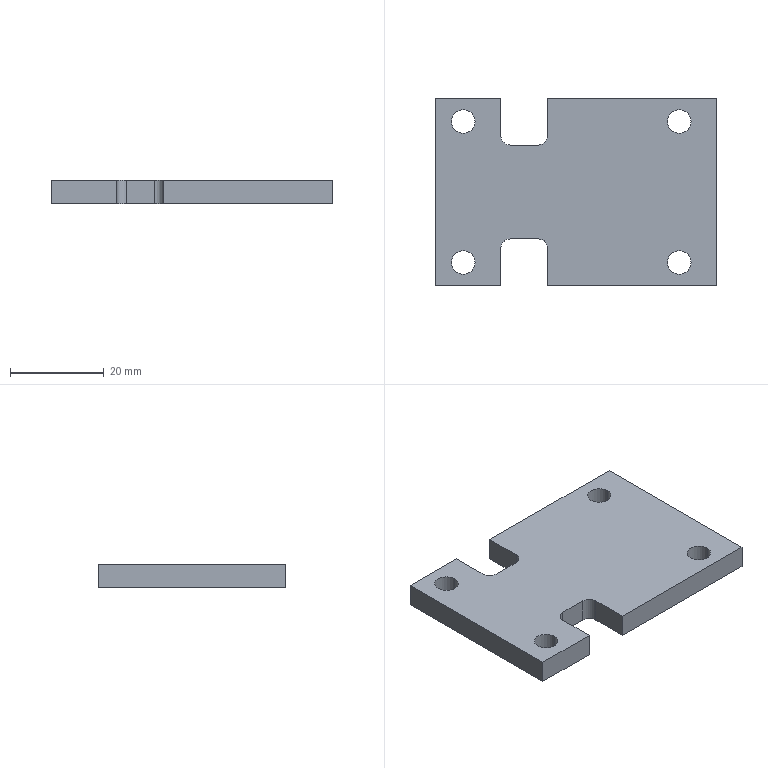Part | NX | 1 solid | 26 faces | box 60 x 40 x 5 mm | volume 10624 mm3 | plane 14 | cylinder 12 | commonest cylinder face diameters 5 x8 4 x4
STEP:
#1=CARTESIAN_POINT('',(-14.,-10.,-2.5));
#2=VERTEX_POINT('',#1);
#3=CARTESIAN_POINT('',(-8.,-10.,-2.5));
#4=VERTEX_POINT('',#3);
#5=CARTESIAN_POINT('',(-14.,-10.,-2.5));
#6=DIRECTION('',(1.,0.,0.));
#7=VECTOR('',#6,1000.);
#8=LINE('',#5,#7);
#9=EDGE_CURVE('',#2,#4,#8,.T.);
#10=ORIENTED_EDGE('',*,*,#9,.F.);
#11=CARTESIAN_POINT('',(-16.,-12.,-2.5));
#12=VERTEX_POINT('',#11);
#13=CARTESIAN_POINT('',(-14.,-12.,-2.5));
#14=DIRECTION('',(0.,0.,-1.));
#15=DIRECTION('',(-1.,0.,0.));
#16=AXIS2_PLACEMENT_3D('',#13,#14,#15);
#17=CIRCLE('',#16,2.);
#18=EDGE_CURVE('',#12,#2,#17,.T.);
#19=ORIENTED_EDGE('',*,*,#18,.F.);
#20=CARTESIAN_POINT('',(-16.,-20.,-2.5));
#21=VERTEX_POINT('',#20);
#22=CARTESIAN_POINT('',(-16.,-12.,-2.5));
#23=DIRECTION('',(0.,-1.,0.));
#24=VECTOR('',#23,1000.);
#25=LINE('',#22,#24);
#26=EDGE_CURVE('',#12,#21,#25,.T.);
#27=ORIENTED_EDGE('',*,*,#26,.T.);
#28=CARTESIAN_POINT('',(-30.,-20.,-2.5));
#29=VERTEX_POINT('',#28);
#30=CARTESIAN_POINT('',(-16.,-20.,-2.5));
#31=DIRECTION('',(-1.,0.,0.));
#32=VECTOR('',#31,1000.);
#33=LINE('',#30,#32);
#34=EDGE_CURVE('',#21,#29,#33,.T.);
#35=ORIENTED_EDGE('',*,*,#34,.T.);
#36=CARTESIAN_POINT('',(-30.,20.,-2.5));
#37=VERTEX_POINT('',#36);
#38=CARTESIAN_POINT('',(-30.,-20.,-2.5));
#39=DIRECTION('',(0.,1.,0.));
#40=VECTOR('',#39,1000.);
#41=LINE('',#38,#40);
#42=EDGE_CURVE('',#29,#37,#41,.T.);
#43=ORIENTED_EDGE('',*,*,#42,.T.);
#44=CARTESIAN_POINT('',(-16.,20.,-2.5));
#45=VERTEX_POINT('',#44);
#46=CARTESIAN_POINT('',(-30.,20.,-2.5));
#47=DIRECTION('',(1.,0.,0.));
#48=VECTOR('',#47,1000.);
#49=LINE('',#46,#48);
#50=EDGE_CURVE('',#37,#45,#49,.T.);
#51=ORIENTED_EDGE('',*,*,#50,.T.);
#52=CARTESIAN_POINT('',(-16.,12.,-2.5));
#53=VERTEX_POINT('',#52);
#54=CARTESIAN_POINT('',(-16.,12.,-2.5));
#55=DIRECTION('',(0.,1.,0.));
#56=VECTOR('',#55,1000.);
#57=LINE('',#54,#56);
#58=EDGE_CURVE('',#53,#45,#57,.T.);
#59=ORIENTED_EDGE('',*,*,#58,.F.);
#60=CARTESIAN_POINT('',(-14.,10.,-2.5));
#61=VERTEX_POINT('',#60);
#62=CARTESIAN_POINT('',(-14.,12.,-2.5));
#63=DIRECTION('',(0.,0.,-1.));
#64=DIRECTION('',(0.,-1.,0.));
#65=AXIS2_PLACEMENT_3D('',#62,#63,#64);
#66=CIRCLE('',#65,2.);
#67=EDGE_CURVE('',#61,#53,#66,.T.);
#68=ORIENTED_EDGE('',*,*,#67,.F.);
#69=CARTESIAN_POINT('',(-8.,10.,-2.5));
#70=VERTEX_POINT('',#69);
#71=CARTESIAN_POINT('',(-8.,10.,-2.5));
#72=DIRECTION('',(-1.,0.,0.));
#73=VECTOR('',#72,1000.);
#74=LINE('',#71,#73);
#75=EDGE_CURVE('',#70,#61,#74,.T.);
#76=ORIENTED_EDGE('',*,*,#75,.F.);
#77=CARTESIAN_POINT('',(-6.,12.,-2.5));
#78=VERTEX_POINT('',#77);
#79=CARTESIAN_POINT('',(-8.,12.,-2.5));
#80=DIRECTION('',(0.,0.,-1.));
#81=DIRECTION('',(1.,0.,0.));
#82=AXIS2_PLACEMENT_3D('',#79,#80,#81);
#83=CIRCLE('',#82,2.);
#84=EDGE_CURVE('',#78,#70,#83,.T.);
#85=ORIENTED_EDGE('',*,*,#84,.F.);
#86=CARTESIAN_POINT('',(-6.,20.,-2.5));
#87=VERTEX_POINT('',#86);
#88=CARTESIAN_POINT('',(-6.,12.,-2.5));
#89=DIRECTION('',(0.,1.,0.));
#90=VECTOR('',#89,1000.);
#91=LINE('',#88,#90);
#92=EDGE_CURVE('',#78,#87,#91,.T.);
#93=ORIENTED_EDGE('',*,*,#92,.T.);
#94=CARTESIAN_POINT('',(30.,20.,-2.5));
#95=VERTEX_POINT('',#94);
#96=CARTESIAN_POINT('',(-6.,20.,-2.5));
#97=DIRECTION('',(1.,0.,0.));
#98=VECTOR('',#97,1000.);
#99=LINE('',#96,#98);
#100=EDGE_CURVE('',#87,#95,#99,.T.);
#101=ORIENTED_EDGE('',*,*,#100,.T.);
#102=CARTESIAN_POINT('',(30.,-20.,-2.5));
#103=VERTEX_POINT('',#102);
#104=CARTESIAN_POINT('',(30.,20.,-2.5));
#105=DIRECTION('',(0.,-1.,0.));
#106=VECTOR('',#105,1000.);
#107=LINE('',#104,#106);
#108=EDGE_CURVE('',#95,#103,#107,.T.);
#109=ORIENTED_EDGE('',*,*,#108,.T.);
#110=CARTESIAN_POINT('',(-6.,-20.,-2.5));
#111=VERTEX_POINT('',#110);
#112=CARTESIAN_POINT('',(30.,-20.,-2.5));
#113=DIRECTION('',(-1.,0.,0.));
#114=VECTOR('',#113,1000.);
#115=LINE('',#112,#114);
#116=EDGE_CURVE('',#103,#111,#115,.T.);
#117=ORIENTED_EDGE('',*,*,#116,.T.);
#118=CARTESIAN_POINT('',(-6.,-12.,-2.5));
#119=VERTEX_POINT('',#118);
#120=CARTESIAN_POINT('',(-6.,-12.,-2.5));
#121=DIRECTION('',(0.,-1.,0.));
#122=VECTOR('',#121,1000.);
#123=LINE('',#120,#122);
#124=EDGE_CURVE('',#119,#111,#123,.T.);
#125=ORIENTED_EDGE('',*,*,#124,.F.);
#126=CARTESIAN_POINT('',(-8.,-12.,-2.5));
#127=DIRECTION('',(0.,0.,-1.));
#128=DIRECTION('',(0.,1.,0.));
#129=AXIS2_PLACEMENT_3D('',#126,#127,#128);
#130=CIRCLE('',#129,2.);
#131=EDGE_CURVE('',#4,#119,#130,.T.);
#132=ORIENTED_EDGE('',*,*,#131,.F.);
#133=EDGE_LOOP('',(#10,#19,#27,#35,#43,#51,#59,#68,#76,#85,#93,#101,#109,#117,#125,#132));
#134=FACE_BOUND('',#133,.T.);
#135=CARTESIAN_POINT('',(-26.5,-15.,-2.5));
#136=VERTEX_POINT('',#135);
#137=CARTESIAN_POINT('',(-21.5,-15.,-2.5));
#138=VERTEX_POINT('',#137);
#139=CARTESIAN_POINT('',(-24.,-15.,-2.5));
#140=DIRECTION('',(0.,0.,-1.));
#141=DIRECTION('',(1.,0.,0.));
#142=AXIS2_PLACEMENT_3D('',#139,#140,#141);
#143=CIRCLE('',#142,2.5);
#144=EDGE_CURVE('',#136,#138,#143,.T.);
#145=ORIENTED_EDGE('',*,*,#144,.F.);
#146=CARTESIAN_POINT('',(-24.,-15.,-2.5));
#147=DIRECTION('',(0.,0.,-1.));
#148=DIRECTION('',(1.,0.,0.));
#149=AXIS2_PLACEMENT_3D('',#146,#147,#148);
#150=CIRCLE('',#149,2.5);
#151=EDGE_CURVE('',#138,#136,#150,.T.);
#152=ORIENTED_EDGE('',*,*,#151,.F.);
#153=EDGE_LOOP('',(#145,#152));
#154=FACE_BOUND('',#153,.T.);
#155=CARTESIAN_POINT('',(24.5,-15.,-2.5));
#156=VERTEX_POINT('',#155);
#157=CARTESIAN_POINT('',(19.5,-15.,-2.5));
#158=VERTEX_POINT('',#157);
#159=CARTESIAN_POINT('',(22.,-15.,-2.5));
#160=DIRECTION('',(0.,0.,-1.));
#161=DIRECTION('',(1.,0.,0.));
#162=AXIS2_PLACEMENT_3D('',#159,#160,#161);
#163=CIRCLE('',#162,2.5);
#164=EDGE_CURVE('',#156,#158,#163,.T.);
#165=ORIENTED_EDGE('',*,*,#164,.F.);
#166=CARTESIAN_POINT('',(22.,-15.,-2.5));
#167=DIRECTION('',(0.,0.,-1.));
#168=DIRECTION('',(1.,0.,0.));
#169=AXIS2_PLACEMENT_3D('',#166,#167,#168);
#170=CIRCLE('',#169,2.5);
#171=EDGE_CURVE('',#158,#156,#170,.T.);
#172=ORIENTED_EDGE('',*,*,#171,.F.);
#173=EDGE_LOOP('',(#165,#172));
#174=FACE_BOUND('',#173,.T.);
#175=CARTESIAN_POINT('',(24.5,15.,-2.5));
#176=VERTEX_POINT('',#175);
#177=CARTESIAN_POINT('',(19.5,15.,-2.5));
#178=VERTEX_POINT('',#177);
#179=CARTESIAN_POINT('',(22.,15.,-2.5));
#180=DIRECTION('',(0.,0.,-1.));
#181=DIRECTION('',(1.,0.,0.));
#182=AXIS2_PLACEMENT_3D('',#179,#180,#181);
#183=CIRCLE('',#182,2.5);
#184=EDGE_CURVE('',#176,#178,#183,.T.);
#185=ORIENTED_EDGE('',*,*,#184,.F.);
#186=CARTESIAN_POINT('',(22.,15.,-2.5));
#187=DIRECTION('',(0.,0.,-1.));
#188=DIRECTION('',(1.,0.,0.));
#189=AXIS2_PLACEMENT_3D('',#186,#187,#188);
#190=CIRCLE('',#189,2.5);
#191=EDGE_CURVE('',#178,#176,#190,.T.);
#192=ORIENTED_EDGE('',*,*,#191,.F.);
#193=EDGE_LOOP('',(#185,#192));
#194=FACE_BOUND('',#193,.T.);
#195=CARTESIAN_POINT('',(-21.5,15.,-2.5));
#196=VERTEX_POINT('',#195);
#197=CARTESIAN_POINT('',(-26.5,15.,-2.5));
#198=VERTEX_POINT('',#197);
#199=CARTESIAN_POINT('',(-24.,15.,-2.5));
#200=DIRECTION('',(0.,0.,-1.));
#201=DIRECTION('',(1.,0.,0.));
#202=AXIS2_PLACEMENT_3D('',#199,#200,#201);
#203=CIRCLE('',#202,2.5);
#204=EDGE_CURVE('',#196,#198,#203,.T.);
#205=ORIENTED_EDGE('',*,*,#204,.F.);
#206=CARTESIAN_POINT('',(-24.,15.,-2.5));
#207=DIRECTION('',(0.,0.,-1.));
#208=DIRECTION('',(1.,0.,0.));
#209=AXIS2_PLACEMENT_3D('',#206,#207,#208);
#210=CIRCLE('',#209,2.5);
#211=EDGE_CURVE('',#198,#196,#210,.T.);
#212=ORIENTED_EDGE('',*,*,#211,.F.);
#213=EDGE_LOOP('',(#205,#212));
#214=FACE_BOUND('',#213,.T.);
#215=CARTESIAN_POINT('',(0.,0.,-2.5));
#216=DIRECTION('',(0.,0.,1.));
#217=DIRECTION('',(1.,0.,0.));
#218=AXIS2_PLACEMENT_3D('',#215,#216,#217);
#219=PLANE('',#218);
#220=ADVANCED_FACE('',(#134,#154,#174,#194,#214),#219,.F.);
#221=CARTESIAN_POINT('',(-14.,-10.,2.5));
#222=VERTEX_POINT('',#221);
#223=CARTESIAN_POINT('',(-14.,-10.,2.5));
#224=DIRECTION('',(0.,0.,-1.));
#225=VECTOR('',#224,1000.);
#226=LINE('',#223,#225);
#227=EDGE_CURVE('',#222,#2,#226,.T.);
#228=ORIENTED_EDGE('',*,*,#227,.T.);
#229=ORIENTED_EDGE('',*,*,#9,.T.);
#230=CARTESIAN_POINT('',(-8.,-10.,2.5));
#231=VERTEX_POINT('',#230);
#232=CARTESIAN_POINT('',(-8.,-10.,2.624));
#233=DIRECTION('',(0.,0.,-1.));
#234=VECTOR('',#233,1000.);
#235=LINE('',#232,#234);
#236=EDGE_CURVE('',#231,#4,#235,.T.);
#237=ORIENTED_EDGE('',*,*,#236,.F.);
#238=CARTESIAN_POINT('',(-14.,-10.,2.5));
#239=DIRECTION('',(1.,0.,0.));
#240=VECTOR('',#239,1000.);
#241=LINE('',#238,#240);
#242=EDGE_CURVE('',#222,#231,#241,.T.);
#243=ORIENTED_EDGE('',*,*,#242,.F.);
#244=EDGE_LOOP('',(#228,#229,#237,#243));
#245=FACE_BOUND('',#244,.T.);
#246=CARTESIAN_POINT('',(-6.,-10.,2.5));
#247=DIRECTION('',(0.,1.,0.));
#248=DIRECTION('',(1.,0.,0.));
#249=AXIS2_PLACEMENT_3D('',#246,#247,#248);
#250=PLANE('',#249);
#251=ADVANCED_FACE('',(#245),#250,.F.);
#252=CARTESIAN_POINT('',(-16.,-12.,2.5));
#253=VERTEX_POINT('',#252);
#254=CARTESIAN_POINT('',(-16.,-12.,2.624));
#255=DIRECTION('',(0.,0.,-1.));
#256=VECTOR('',#255,1000.);
#257=LINE('',#254,#256);
#258=EDGE_CURVE('',#253,#12,#257,.T.);
#259=ORIENTED_EDGE('',*,*,#258,.T.);
#260=ORIENTED_EDGE('',*,*,#18,.T.);
#261=ORIENTED_EDGE('',*,*,#227,.F.);
#262=CARTESIAN_POINT('',(-14.,-12.,2.5));
#263=DIRECTION('',(0.,0.,1.));
#264=DIRECTION('',(0.,1.,0.));
#265=AXIS2_PLACEMENT_3D('',#262,#263,#264);
#266=CIRCLE('',#265,2.);
#267=EDGE_CURVE('',#222,#253,#266,.T.);
#268=ORIENTED_EDGE('',*,*,#267,.T.);
#269=EDGE_LOOP('',(#259,#260,#261,#268));
#270=FACE_BOUND('',#269,.T.);
#271=CARTESIAN_POINT('',(-14.,-12.,2.624));
#272=DIRECTION('',(0.,0.,-1.));
#273=DIRECTION('',(-1.,0.,0.));
#274=AXIS2_PLACEMENT_3D('',#271,#272,#273);
#275=CYLINDRICAL_SURFACE('',#274,2.);
#276=ADVANCED_FACE('',(#270),#275,.F.);
#277=ORIENTED_EDGE('',*,*,#258,.F.);
#278=CARTESIAN_POINT('',(-16.,-20.,2.5));
#279=VERTEX_POINT('',#278);
#280=CARTESIAN_POINT('',(-16.,-12.,2.5));
#281=DIRECTION('',(0.,-1.,0.));
#282=VECTOR('',#281,1000.);
#283=LINE('',#280,#282);
#284=EDGE_CURVE('',#253,#279,#283,.T.);
#285=ORIENTED_EDGE('',*,*,#284,.T.);
#286=CARTESIAN_POINT('',(-16.,-20.,2.5));
#287=DIRECTION('',(0.,0.,-1.));
#288=VECTOR('',#287,1000.);
#289=LINE('',#286,#288);
#290=EDGE_CURVE('',#279,#21,#289,.T.);
#291=ORIENTED_EDGE('',*,*,#290,.T.);
#292=ORIENTED_EDGE('',*,*,#26,.F.);
#293=EDGE_LOOP('',(#277,#285,#291,#292));
#294=FACE_BOUND('',#293,.T.);
#295=CARTESIAN_POINT('',(-16.,-10.,2.5));
#296=DIRECTION('',(-1.,0.,0.));
#297=DIRECTION('',(0.,0.,1.));
#298=AXIS2_PLACEMENT_3D('',#295,#296,#297);
#299=PLANE('',#298);
#300=ADVANCED_FACE('',(#294),#299,.F.);
#301=ORIENTED_EDGE('',*,*,#290,.F.);
#302=CARTESIAN_POINT('',(-30.,-20.,2.5));
#303=VERTEX_POINT('',#302);
#304=CARTESIAN_POINT('',(-16.,-20.,2.5));
#305=DIRECTION('',(-1.,0.,0.));
#306=VECTOR('',#305,1000.);
#307=LINE('',#304,#306);
#308=EDGE_CURVE('',#279,#303,#307,.T.);
#309=ORIENTED_EDGE('',*,*,#308,.T.);
#310=CARTESIAN_POINT('',(-30.,-20.,2.5));
#311=DIRECTION('',(0.,0.,-1.));
#312=VECTOR('',#311,1000.);
#313=LINE('',#310,#312);
#314=EDGE_CURVE('',#303,#29,#313,.T.);
#315=ORIENTED_EDGE('',*,*,#314,.T.);
#316=ORIENTED_EDGE('',*,*,#34,.F.);
#317=EDGE_LOOP('',(#301,#309,#315,#316));
#318=FACE_BOUND('',#317,.T.);
#319=CARTESIAN_POINT('',(-30.,-20.,-2.5));
#320=DIRECTION('',(0.,-1.,0.));
#321=DIRECTION('',(0.,0.,-1.));
#322=AXIS2_PLACEMENT_3D('',#319,#320,#321);
#323=PLANE('',#322);
#324=ADVANCED_FACE('',(#318),#323,.T.);
#325=ORIENTED_EDGE('',*,*,#42,.F.);
#326=ORIENTED_EDGE('',*,*,#314,.F.);
#327=CARTESIAN_POINT('',(-30.,20.,2.5));
#328=VERTEX_POINT('',#327);
#329=CARTESIAN_POINT('',(-30.,-20.,2.5));
#330=DIRECTION('',(0.,1.,0.));
#331=VECTOR('',#330,1000.);
#332=LINE('',#329,#331);
#333=EDGE_CURVE('',#303,#328,#332,.T.);
#334=ORIENTED_EDGE('',*,*,#333,.T.);
#335=CARTESIAN_POINT('',(-30.,20.,2.5));
#336=DIRECTION('',(0.,0.,-1.));
#337=VECTOR('',#336,1000.);
#338=LINE('',#335,#337);
#339=EDGE_CURVE('',#328,#37,#338,.T.);
#340=ORIENTED_EDGE('',*,*,#339,.T.);
#341=EDGE_LOOP('',(#325,#326,#334,#340));
#342=FACE_BOUND('',#341,.T.);
#343=CARTESIAN_POINT('',(-30.,20.,-2.5));
#344=DIRECTION('',(-1.,0.,0.));
#345=DIRECTION('',(0.,0.,1.));
#346=AXIS2_PLACEMENT_3D('',#343,#344,#345);
#347=PLANE('',#346);
#348=ADVANCED_FACE('',(#342),#347,.T.);
#349=CARTESIAN_POINT('',(-16.,20.,2.5));
#350=VERTEX_POINT('',#349);
#351=CARTESIAN_POINT('',(-16.,20.,2.5));
#352=DIRECTION('',(0.,0.,-1.));
#353=VECTOR('',#352,1000.);
#354=LINE('',#351,#353);
#355=EDGE_CURVE('',#350,#45,#354,.T.);
#356=ORIENTED_EDGE('',*,*,#355,.T.);
#357=ORIENTED_EDGE('',*,*,#50,.F.);
#358=ORIENTED_EDGE('',*,*,#339,.F.);
#359=CARTESIAN_POINT('',(-30.,20.,2.5));
#360=DIRECTION('',(1.,0.,0.));
#361=VECTOR('',#360,1000.);
#362=LINE('',#359,#361);
#363=EDGE_CURVE('',#328,#350,#362,.T.);
#364=ORIENTED_EDGE('',*,*,#363,.T.);
#365=EDGE_LOOP('',(#356,#357,#358,#364));
#366=FACE_BOUND('',#365,.T.);
#367=CARTESIAN_POINT('',(30.,20.,-2.5));
#368=DIRECTION('',(0.,1.,0.));
#369=DIRECTION('',(1.,0.,0.));
#370=AXIS2_PLACEMENT_3D('',#367,#368,#369);
#371=PLANE('',#370);
#372=ADVANCED_FACE('',(#366),#371,.T.);
#373=CARTESIAN_POINT('',(-16.,12.,2.5));
#374=VERTEX_POINT('',#373);
#375=CARTESIAN_POINT('',(-16.,12.,2.5));
#376=DIRECTION('',(0.,0.,-1.));
#377=VECTOR('',#376,1000.);
#378=LINE('',#375,#377);
#379=EDGE_CURVE('',#374,#53,#378,.T.);
#380=ORIENTED_EDGE('',*,*,#379,.T.);
#381=ORIENTED_EDGE('',*,*,#58,.T.);
#382=ORIENTED_EDGE('',*,*,#355,.F.);
#383=CARTESIAN_POINT('',(-16.,12.,2.5));
#384=DIRECTION('',(0.,1.,0.));
#385=VECTOR('',#384,1000.);
#386=LINE('',#383,#385);
#387=EDGE_CURVE('',#374,#350,#386,.T.);
#388=ORIENTED_EDGE('',*,*,#387,.F.);
#389=EDGE_LOOP('',(#380,#381,#382,#388));
#390=FACE_BOUND('',#389,.T.);
#391=CARTESIAN_POINT('',(-16.,20.,2.5));
#392=DIRECTION('',(-1.,0.,0.));
#393=DIRECTION('',(0.,0.,1.));
#394=AXIS2_PLACEMENT_3D('',#391,#392,#393);
#395=PLANE('',#394);
#396=ADVANCED_FACE('',(#390),#395,.F.);
#397=CARTESIAN_POINT('',(-14.,10.,2.5));
#398=VERTEX_POINT('',#397);
#399=CARTESIAN_POINT('',(-14.,10.,2.624));
#400=DIRECTION('',(0.,0.,-1.));
#401=VECTOR('',#400,1000.);
#402=LINE('',#399,#401);
#403=EDGE_CURVE('',#398,#61,#402,.T.);
#404=ORIENTED_EDGE('',*,*,#403,.T.);
#405=ORIENTED_EDGE('',*,*,#67,.T.);
#406=ORIENTED_EDGE('',*,*,#379,.F.);
#407=CARTESIAN_POINT('',(-14.,12.,2.5));
#408=DIRECTION('',(0.,0.,1.));
#409=DIRECTION('',(-1.,0.,0.));
#410=AXIS2_PLACEMENT_3D('',#407,#408,#409);
#411=CIRCLE('',#410,2.);
#412=EDGE_CURVE('',#374,#398,#411,.T.);
#413=ORIENTED_EDGE('',*,*,#412,.T.);
#414=EDGE_LOOP('',(#404,#405,#406,#413));
#415=FACE_BOUND('',#414,.T.);
#416=CARTESIAN_POINT('',(-14.,12.,2.624));
#417=DIRECTION('',(0.,0.,-1.));
#418=DIRECTION('',(0.,-1.,0.));
#419=AXIS2_PLACEMENT_3D('',#416,#417,#418);
#420=CYLINDRICAL_SURFACE('',#419,2.);
#421=ADVANCED_FACE('',(#415),#420,.F.);
#422=CARTESIAN_POINT('',(-8.,10.,2.5));
#423=VERTEX_POINT('',#422);
#424=CARTESIAN_POINT('',(-8.,10.,2.5));
#425=DIRECTION('',(0.,0.,-1.));
#426=VECTOR('',#425,1000.);
#427=LINE('',#424,#426);
#428=EDGE_CURVE('',#423,#70,#427,.T.);
#429=ORIENTED_EDGE('',*,*,#428,.T.);
#430=ORIENTED_EDGE('',*,*,#75,.T.);
#431=ORIENTED_EDGE('',*,*,#403,.F.);
#432=CARTESIAN_POINT('',(-8.,10.,2.5));
#433=DIRECTION('',(-1.,0.,0.));
#434=VECTOR('',#433,1000.);
#435=LINE('',#432,#434);
#436=EDGE_CURVE('',#423,#398,#435,.T.);
#437=ORIENTED_EDGE('',*,*,#436,.F.);
#438=EDGE_LOOP('',(#429,#430,#431,#437));
#439=FACE_BOUND('',#438,.T.);
#440=CARTESIAN_POINT('',(-16.,10.,2.5));
#441=DIRECTION('',(0.,-1.,0.));
#442=DIRECTION('',(0.,0.,-1.));
#443=AXIS2_PLACEMENT_3D('',#440,#441,#442);
#444=PLANE('',#443);
#445=ADVANCED_FACE('',(#439),#444,.F.);
#446=CARTESIAN_POINT('',(-6.,12.,2.5));
#447=VERTEX_POINT('',#446);
#448=CARTESIAN_POINT('',(-6.,12.,2.624));
#449=DIRECTION('',(0.,0.,-1.));
#450=VECTOR('',#449,1000.);
#451=LINE('',#448,#450);
#452=EDGE_CURVE('',#447,#78,#451,.T.);
#453=ORIENTED_EDGE('',*,*,#452,.T.);
#454=ORIENTED_EDGE('',*,*,#84,.T.);
#455=ORIENTED_EDGE('',*,*,#428,.F.);
#456=CARTESIAN_POINT('',(-8.,12.,2.5));
#457=DIRECTION('',(0.,0.,1.));
#458=DIRECTION('',(0.,-1.,0.));
#459=AXIS2_PLACEMENT_3D('',#456,#457,#458);
#460=CIRCLE('',#459,2.);
#461=EDGE_CURVE('',#423,#447,#460,.T.);
#462=ORIENTED_EDGE('',*,*,#461,.T.);
#463=EDGE_LOOP('',(#453,#454,#455,#462));
#464=FACE_BOUND('',#463,.T.);
#465=CARTESIAN_POINT('',(-8.,12.,2.624));
#466=DIRECTION('',(0.,0.,-1.));
#467=DIRECTION('',(1.,0.,0.));
#468=AXIS2_PLACEMENT_3D('',#465,#466,#467);
#469=CYLINDRICAL_SURFACE('',#468,2.);
#470=ADVANCED_FACE('',(#464),#469,.F.);
#471=ORIENTED_EDGE('',*,*,#452,.F.);
#472=CARTESIAN_POINT('',(-6.,20.,2.5));
#473=VERTEX_POINT('',#472);
#474=CARTESIAN_POINT('',(-6.,12.,2.5));
#475=DIRECTION('',(0.,1.,0.));
#476=VECTOR('',#475,1000.);
#477=LINE('',#474,#476);
#478=EDGE_CURVE('',#447,#473,#477,.T.);
#479=ORIENTED_EDGE('',*,*,#478,.T.);
#480=CARTESIAN_POINT('',(-6.,20.,2.5));
#481=DIRECTION('',(0.,0.,-1.));
#482=VECTOR('',#481,1000.);
#483=LINE('',#480,#482);
#484=EDGE_CURVE('',#473,#87,#483,.T.);
#485=ORIENTED_EDGE('',*,*,#484,.T.);
#486=ORIENTED_EDGE('',*,*,#92,.F.);
#487=EDGE_LOOP('',(#471,#479,#485,#486));
#488=FACE_BOUND('',#487,.T.);
#489=CARTESIAN_POINT('',(-6.,10.,2.5));
#490=DIRECTION('',(1.,0.,0.));
#491=DIRECTION('',(0.,1.,0.));
#492=AXIS2_PLACEMENT_3D('',#489,#490,#491);
#493=PLANE('',#492);
#494=ADVANCED_FACE('',(#488),#493,.F.);
#495=ORIENTED_EDGE('',*,*,#484,.F.);
#496=CARTESIAN_POINT('',(30.,20.,2.5));
#497=VERTEX_POINT('',#496);
#498=CARTESIAN_POINT('',(-6.,20.,2.5));
#499=DIRECTION('',(1.,0.,0.));
#500=VECTOR('',#499,1000.);
#501=LINE('',#498,#500);
#502=EDGE_CURVE('',#473,#497,#501,.T.);
#503=ORIENTED_EDGE('',*,*,#502,.T.);
#504=CARTESIAN_POINT('',(30.,20.,2.5));
#505=DIRECTION('',(0.,0.,-1.));
#506=VECTOR('',#505,1000.);
#507=LINE('',#504,#506);
#508=EDGE_CURVE('',#497,#95,#507,.T.);
#509=ORIENTED_EDGE('',*,*,#508,.T.);
#510=ORIENTED_EDGE('',*,*,#100,.F.);
#511=EDGE_LOOP('',(#495,#503,#509,#510));
#512=FACE_BOUND('',#511,.T.);
#513=CARTESIAN_POINT('',(30.,20.,-2.5));
#514=DIRECTION('',(0.,1.,0.));
#515=DIRECTION('',(1.,0.,0.));
#516=AXIS2_PLACEMENT_3D('',#513,#514,#515);
#517=PLANE('',#516);
#518=ADVANCED_FACE('',(#512),#517,.T.);
#519=ORIENTED_EDGE('',*,*,#108,.F.);
#520=ORIENTED_EDGE('',*,*,#508,.F.);
#521=CARTESIAN_POINT('',(30.,-20.,2.5));
#522=VERTEX_POINT('',#521);
#523=CARTESIAN_POINT('',(30.,20.,2.5));
#524=DIRECTION('',(0.,-1.,0.));
#525=VECTOR('',#524,1000.);
#526=LINE('',#523,#525);
#527=EDGE_CURVE('',#497,#522,#526,.T.);
#528=ORIENTED_EDGE('',*,*,#527,.T.);
#529=CARTESIAN_POINT('',(30.,-20.,2.5));
#530=DIRECTION('',(0.,0.,-1.));
#531=VECTOR('',#530,1000.);
#532=LINE('',#529,#531);
#533=EDGE_CURVE('',#522,#103,#532,.T.);
#534=ORIENTED_EDGE('',*,*,#533,.T.);
#535=EDGE_LOOP('',(#519,#520,#528,#534));
#536=FACE_BOUND('',#535,.T.);
#537=CARTESIAN_POINT('',(30.,-20.,-2.5));
#538=DIRECTION('',(1.,0.,0.));
#539=DIRECTION('',(0.,1.,0.));
#540=AXIS2_PLACEMENT_3D('',#537,#538,#539);
#541=PLANE('',#540);
#542=ADVANCED_FACE('',(#536),#541,.T.);
#543=CARTESIAN_POINT('',(-6.,-20.,2.5));
#544=VERTEX_POINT('',#543);
#545=CARTESIAN_POINT('',(-6.,-20.,2.5));
#546=DIRECTION('',(0.,0.,-1.));
#547=VECTOR('',#546,1000.);
#548=LINE('',#545,#547);
#549=EDGE_CURVE('',#544,#111,#548,.T.);
#550=ORIENTED_EDGE('',*,*,#549,.T.);
#551=ORIENTED_EDGE('',*,*,#116,.F.);
#552=ORIENTED_EDGE('',*,*,#533,.F.);
#553=CARTESIAN_POINT('',(30.,-20.,2.5));
#554=DIRECTION('',(-1.,0.,0.));
#555=VECTOR('',#554,1000.);
#556=LINE('',#553,#555);
#557=EDGE_CURVE('',#522,#544,#556,.T.);
#558=ORIENTED_EDGE('',*,*,#557,.T.);
#559=EDGE_LOOP('',(#550,#551,#552,#558));
#560=FACE_BOUND('',#559,.T.);
#561=CARTESIAN_POINT('',(-30.,-20.,-2.5));
#562=DIRECTION('',(0.,-1.,0.));
#563=DIRECTION('',(0.,0.,-1.));
#564=AXIS2_PLACEMENT_3D('',#561,#562,#563);
#565=PLANE('',#564);
#566=ADVANCED_FACE('',(#560),#565,.T.);
#567=CARTESIAN_POINT('',(-6.,-12.,2.5));
#568=VERTEX_POINT('',#567);
#569=CARTESIAN_POINT('',(-6.,-12.,2.5));
#570=DIRECTION('',(0.,0.,-1.));
#571=VECTOR('',#570,1000.);
#572=LINE('',#569,#571);
#573=EDGE_CURVE('',#568,#119,#572,.T.);
#574=ORIENTED_EDGE('',*,*,#573,.T.);
#575=ORIENTED_EDGE('',*,*,#124,.T.);
#576=ORIENTED_EDGE('',*,*,#549,.F.);
#577=CARTESIAN_POINT('',(-6.,-12.,2.5));
#578=DIRECTION('',(0.,-1.,0.));
#579=VECTOR('',#578,1000.);
#580=LINE('',#577,#579);
#581=EDGE_CURVE('',#568,#544,#580,.T.);
#582=ORIENTED_EDGE('',*,*,#581,.F.);
#583=EDGE_LOOP('',(#574,#575,#576,#582));
#584=FACE_BOUND('',#583,.T.);
#585=CARTESIAN_POINT('',(-6.,-20.,2.5));
#586=DIRECTION('',(1.,0.,0.));
#587=DIRECTION('',(0.,1.,0.));
#588=AXIS2_PLACEMENT_3D('',#585,#586,#587);
#589=PLANE('',#588);
#590=ADVANCED_FACE('',(#584),#589,.F.);
#591=ORIENTED_EDGE('',*,*,#236,.T.);
#592=ORIENTED_EDGE('',*,*,#131,.T.);
#593=ORIENTED_EDGE('',*,*,#573,.F.);
#594=CARTESIAN_POINT('',(-8.,-12.,2.5));
#595=DIRECTION('',(0.,0.,1.));
#596=DIRECTION('',(1.,0.,0.));
#597=AXIS2_PLACEMENT_3D('',#594,#595,#596);
#598=CIRCLE('',#597,2.);
#599=EDGE_CURVE('',#568,#231,#598,.T.);
#600=ORIENTED_EDGE('',*,*,#599,.T.);
#601=EDGE_LOOP('',(#591,#592,#593,#600));
#602=FACE_BOUND('',#601,.T.);
#603=CARTESIAN_POINT('',(-8.,-12.,2.624));
#604=DIRECTION('',(0.,0.,-1.));
#605=DIRECTION('',(0.,1.,0.));
#606=AXIS2_PLACEMENT_3D('',#603,#604,#605);
#607=CYLINDRICAL_SURFACE('',#606,2.);
#608=ADVANCED_FACE('',(#602),#607,.F.);
#609=ORIENTED_EDGE('',*,*,#581,.T.);
#610=ORIENTED_EDGE('',*,*,#557,.F.);
#611=ORIENTED_EDGE('',*,*,#527,.F.);
#612=ORIENTED_EDGE('',*,*,#502,.F.);
#613=ORIENTED_EDGE('',*,*,#478,.F.);
#614=ORIENTED_EDGE('',*,*,#461,.F.);
#615=ORIENTED_EDGE('',*,*,#436,.T.);
#616=ORIENTED_EDGE('',*,*,#412,.F.);
#617=ORIENTED_EDGE('',*,*,#387,.T.);
#618=ORIENTED_EDGE('',*,*,#363,.F.);
#619=ORIENTED_EDGE('',*,*,#333,.F.);
#620=ORIENTED_EDGE('',*,*,#308,.F.);
#621=ORIENTED_EDGE('',*,*,#284,.F.);
#622=ORIENTED_EDGE('',*,*,#267,.F.);
#623=ORIENTED_EDGE('',*,*,#242,.T.);
#624=ORIENTED_EDGE('',*,*,#599,.F.);
#625=EDGE_LOOP('',(#609,#610,#611,#612,#613,#614,#615,#616,#617,#618,#619,#620,#621,#622,#623,#624));
#626=FACE_BOUND('',#625,.T.);
#627=CARTESIAN_POINT('',(-26.5,-15.,2.5));
#628=VERTEX_POINT('',#627);
#629=CARTESIAN_POINT('',(-21.5,-15.,2.5));
#630=VERTEX_POINT('',#629);
#631=CARTESIAN_POINT('',(-24.,-15.,2.5));
#632=DIRECTION('',(0.,0.,1.));
#633=DIRECTION('',(-1.,0.,0.));
#634=AXIS2_PLACEMENT_3D('',#631,#632,#633);
#635=CIRCLE('',#634,2.5);
#636=EDGE_CURVE('',#628,#630,#635,.T.);
#637=ORIENTED_EDGE('',*,*,#636,.F.);
#638=CARTESIAN_POINT('',(-24.,-15.,2.5));
#639=DIRECTION('',(0.,0.,1.));
#640=DIRECTION('',(-1.,0.,0.));
#641=AXIS2_PLACEMENT_3D('',#638,#639,#640);
#642=CIRCLE('',#641,2.5);
#643=EDGE_CURVE('',#630,#628,#642,.T.);
#644=ORIENTED_EDGE('',*,*,#643,.F.);
#645=EDGE_LOOP('',(#637,#644));
#646=FACE_BOUND('',#645,.T.);
#647=CARTESIAN_POINT('',(19.5,-15.,2.5));
#648=VERTEX_POINT('',#647);
#649=CARTESIAN_POINT('',(24.5,-15.,2.5));
#650=VERTEX_POINT('',#649);
#651=CARTESIAN_POINT('',(22.,-15.,2.5));
#652=DIRECTION('',(0.,0.,1.));
#653=DIRECTION('',(-1.,0.,0.));
#654=AXIS2_PLACEMENT_3D('',#651,#652,#653);
#655=CIRCLE('',#654,2.5);
#656=EDGE_CURVE('',#648,#650,#655,.T.);
#657=ORIENTED_EDGE('',*,*,#656,.F.);
#658=CARTESIAN_POINT('',(22.,-15.,2.5));
#659=DIRECTION('',(0.,0.,1.));
#660=DIRECTION('',(-1.,0.,0.));
#661=AXIS2_PLACEMENT_3D('',#658,#659,#660);
#662=CIRCLE('',#661,2.5);
#663=EDGE_CURVE('',#650,#648,#662,.T.);
#664=ORIENTED_EDGE('',*,*,#663,.F.);
#665=EDGE_LOOP('',(#657,#664));
#666=FACE_BOUND('',#665,.T.);
#667=CARTESIAN_POINT('',(19.5,15.,2.5));
#668=VERTEX_POINT('',#667);
#669=CARTESIAN_POINT('',(24.5,15.,2.5));
#670=VERTEX_POINT('',#669);
#671=CARTESIAN_POINT('',(22.,15.,2.5));
#672=DIRECTION('',(0.,0.,1.));
#673=DIRECTION('',(-1.,0.,0.));
#674=AXIS2_PLACEMENT_3D('',#671,#672,#673);
#675=CIRCLE('',#674,2.5);
#676=EDGE_CURVE('',#668,#670,#675,.T.);
#677=ORIENTED_EDGE('',*,*,#676,.F.);
#678=CARTESIAN_POINT('',(22.,15.,2.5));
#679=DIRECTION('',(0.,0.,1.));
#680=DIRECTION('',(-1.,0.,0.));
#681=AXIS2_PLACEMENT_3D('',#678,#679,#680);
#682=CIRCLE('',#681,2.5);
#683=EDGE_CURVE('',#670,#668,#682,.T.);
#684=ORIENTED_EDGE('',*,*,#683,.F.);
#685=EDGE_LOOP('',(#677,#684));
#686=FACE_BOUND('',#685,.T.);
#687=CARTESIAN_POINT('',(-26.5,15.,2.5));
#688=VERTEX_POINT('',#687);
#689=CARTESIAN_POINT('',(-21.5,15.,2.5));
#690=VERTEX_POINT('',#689);
#691=CARTESIAN_POINT('',(-24.,15.,2.5));
#692=DIRECTION('',(0.,0.,1.));
#693=DIRECTION('',(-1.,0.,0.));
#694=AXIS2_PLACEMENT_3D('',#691,#692,#693);
#695=CIRCLE('',#694,2.5);
#696=EDGE_CURVE('',#688,#690,#695,.T.);
#697=ORIENTED_EDGE('',*,*,#696,.F.);
#698=CARTESIAN_POINT('',(-24.,15.,2.5));
#699=DIRECTION('',(0.,0.,1.));
#700=DIRECTION('',(-1.,0.,0.));
#701=AXIS2_PLACEMENT_3D('',#698,#699,#700);
#702=CIRCLE('',#701,2.5);
#703=EDGE_CURVE('',#690,#688,#702,.T.);
#704=ORIENTED_EDGE('',*,*,#703,.F.);
#705=EDGE_LOOP('',(#697,#704));
#706=FACE_BOUND('',#705,.T.);
#707=CARTESIAN_POINT('',(0.,0.,2.5));
#708=DIRECTION('',(0.,0.,1.));
#709=DIRECTION('',(1.,0.,0.));
#710=AXIS2_PLACEMENT_3D('',#707,#708,#709);
#711=PLANE('',#710);
#712=ADVANCED_FACE('',(#626,#646,#666,#686,#706),#711,.T.);
#713=ORIENTED_EDGE('',*,*,#636,.T.);
#714=CARTESIAN_POINT('',(-21.5,-15.,-2.5));
#715=DIRECTION('',(0.,0.,1.));
#716=VECTOR('',#715,1000.);
#717=LINE('',#714,#716);
#718=EDGE_CURVE('',#138,#630,#717,.T.);
#719=ORIENTED_EDGE('',*,*,#718,.F.);
#720=ORIENTED_EDGE('',*,*,#151,.T.);
#721=CARTESIAN_POINT('',(-26.5,-15.,-2.5));
#722=DIRECTION('',(0.,0.,1.));
#723=VECTOR('',#722,1000.);
#724=LINE('',#721,#723);
#725=EDGE_CURVE('',#136,#628,#724,.T.);
#726=ORIENTED_EDGE('',*,*,#725,.T.);
#727=EDGE_LOOP('',(#713,#719,#720,#726));
#728=FACE_BOUND('',#727,.T.);
#729=CARTESIAN_POINT('',(-24.,-15.,-2.5));
#730=DIRECTION('',(0.,0.,1.));
#731=DIRECTION('',(1.,0.,0.));
#732=AXIS2_PLACEMENT_3D('',#729,#730,#731);
#733=CYLINDRICAL_SURFACE('',#732,2.5);
#734=ADVANCED_FACE('',(#728),#733,.F.);
#735=ORIENTED_EDGE('',*,*,#696,.T.);
#736=CARTESIAN_POINT('',(-21.5,15.,-2.5));
#737=DIRECTION('',(0.,0.,1.));
#738=VECTOR('',#737,1000.);
#739=LINE('',#736,#738);
#740=EDGE_CURVE('',#196,#690,#739,.T.);
#741=ORIENTED_EDGE('',*,*,#740,.F.);
#742=ORIENTED_EDGE('',*,*,#204,.T.);
#743=CARTESIAN_POINT('',(-26.5,15.,-2.5));
#744=DIRECTION('',(0.,0.,1.));
#745=VECTOR('',#744,1000.);
#746=LINE('',#743,#745);
#747=EDGE_CURVE('',#198,#688,#746,.T.);
#748=ORIENTED_EDGE('',*,*,#747,.T.);
#749=EDGE_LOOP('',(#735,#741,#742,#748));
#750=FACE_BOUND('',#749,.T.);
#751=CARTESIAN_POINT('',(-24.,15.,-2.5));
#752=DIRECTION('',(0.,0.,1.));
#753=DIRECTION('',(1.,0.,0.));
#754=AXIS2_PLACEMENT_3D('',#751,#752,#753);
#755=CYLINDRICAL_SURFACE('',#754,2.5);
#756=ADVANCED_FACE('',(#750),#755,.F.);
#757=ORIENTED_EDGE('',*,*,#164,.T.);
#758=CARTESIAN_POINT('',(19.5,-15.,-2.5));
#759=DIRECTION('',(0.,0.,1.));
#760=VECTOR('',#759,1000.);
#761=LINE('',#758,#760);
#762=EDGE_CURVE('',#158,#648,#761,.T.);
#763=ORIENTED_EDGE('',*,*,#762,.T.);
#764=ORIENTED_EDGE('',*,*,#656,.T.);
#765=CARTESIAN_POINT('',(24.5,-15.,-2.5));
#766=DIRECTION('',(0.,0.,1.));
#767=VECTOR('',#766,1000.);
#768=LINE('',#765,#767);
#769=EDGE_CURVE('',#156,#650,#768,.T.);
#770=ORIENTED_EDGE('',*,*,#769,.F.);
#771=EDGE_LOOP('',(#757,#763,#764,#770));
#772=FACE_BOUND('',#771,.T.);
#773=CARTESIAN_POINT('',(22.,-15.,-2.5));
#774=DIRECTION('',(0.,0.,1.));
#775=DIRECTION('',(1.,0.,0.));
#776=AXIS2_PLACEMENT_3D('',#773,#774,#775);
#777=CYLINDRICAL_SURFACE('',#776,2.5);
#778=ADVANCED_FACE('',(#772),#777,.F.);
#779=ORIENTED_EDGE('',*,*,#184,.T.);
#780=CARTESIAN_POINT('',(19.5,15.,-2.5));
#781=DIRECTION('',(0.,0.,1.));
#782=VECTOR('',#781,1000.);
#783=LINE('',#780,#782);
#784=EDGE_CURVE('',#178,#668,#783,.T.);
#785=ORIENTED_EDGE('',*,*,#784,.T.);
#786=ORIENTED_EDGE('',*,*,#676,.T.);
#787=CARTESIAN_POINT('',(24.5,15.,-2.5));
#788=DIRECTION('',(0.,0.,1.));
#789=VECTOR('',#788,1000.);
#790=LINE('',#787,#789);
#791=EDGE_CURVE('',#176,#670,#790,.T.);
#792=ORIENTED_EDGE('',*,*,#791,.F.);
#793=EDGE_LOOP('',(#779,#785,#786,#792));
#794=FACE_BOUND('',#793,.T.);
#795=CARTESIAN_POINT('',(22.,15.,-2.5));
#796=DIRECTION('',(0.,0.,1.));
#797=DIRECTION('',(1.,0.,0.));
#798=AXIS2_PLACEMENT_3D('',#795,#796,#797);
#799=CYLINDRICAL_SURFACE('',#798,2.5);
#800=ADVANCED_FACE('',(#794),#799,.F.);
#801=ORIENTED_EDGE('',*,*,#791,.T.);
#802=ORIENTED_EDGE('',*,*,#683,.T.);
#803=ORIENTED_EDGE('',*,*,#784,.F.);
#804=ORIENTED_EDGE('',*,*,#191,.T.);
#805=EDGE_LOOP('',(#801,#802,#803,#804));
#806=FACE_BOUND('',#805,.T.);
#807=CARTESIAN_POINT('',(22.,15.,-2.5));
#808=DIRECTION('',(0.,0.,1.));
#809=DIRECTION('',(1.,0.,0.));
#810=AXIS2_PLACEMENT_3D('',#807,#808,#809);
#811=CYLINDRICAL_SURFACE('',#810,2.5);
#812=ADVANCED_FACE('',(#806),#811,.F.);
#813=ORIENTED_EDGE('',*,*,#769,.T.);
#814=ORIENTED_EDGE('',*,*,#663,.T.);
#815=ORIENTED_EDGE('',*,*,#762,.F.);
#816=ORIENTED_EDGE('',*,*,#171,.T.);
#817=EDGE_LOOP('',(#813,#814,#815,#816));
#818=FACE_BOUND('',#817,.T.);
#819=CARTESIAN_POINT('',(22.,-15.,-2.5));
#820=DIRECTION('',(0.,0.,1.));
#821=DIRECTION('',(1.,0.,0.));
#822=AXIS2_PLACEMENT_3D('',#819,#820,#821);
#823=CYLINDRICAL_SURFACE('',#822,2.5);
#824=ADVANCED_FACE('',(#818),#823,.F.);
#825=ORIENTED_EDGE('',*,*,#144,.T.);
#826=ORIENTED_EDGE('',*,*,#718,.T.);
#827=ORIENTED_EDGE('',*,*,#643,.T.);
#828=ORIENTED_EDGE('',*,*,#725,.F.);
#829=EDGE_LOOP('',(#825,#826,#827,#828));
#830=FACE_BOUND('',#829,.T.);
#831=CARTESIAN_POINT('',(-24.,-15.,-2.5));
#832=DIRECTION('',(0.,0.,1.));
#833=DIRECTION('',(1.,0.,0.));
#834=AXIS2_PLACEMENT_3D('',#831,#832,#833);
#835=CYLINDRICAL_SURFACE('',#834,2.5);
#836=ADVANCED_FACE('',(#830),#835,.F.);
#837=ORIENTED_EDGE('',*,*,#740,.T.);
#838=ORIENTED_EDGE('',*,*,#703,.T.);
#839=ORIENTED_EDGE('',*,*,#747,.F.);
#840=ORIENTED_EDGE('',*,*,#211,.T.);
#841=EDGE_LOOP('',(#837,#838,#839,#840));
#842=FACE_BOUND('',#841,.T.);
#843=CARTESIAN_POINT('',(-24.,15.,-2.5));
#844=DIRECTION('',(0.,0.,1.));
#845=DIRECTION('',(1.,0.,0.));
#846=AXIS2_PLACEMENT_3D('',#843,#844,#845);
#847=CYLINDRICAL_SURFACE('',#846,2.5);
#848=ADVANCED_FACE('',(#842),#847,.F.);
#849=CLOSED_SHELL('',(#220,#251,#276,#300,#324,#348,#372,#396,#421,#445,#470,#494,#518,#542,#566,#590,#608,#712,#734,#756,#778,#800,#812,#824,#836,#848));
#850=MANIFOLD_SOLID_BREP('',#849);
#851=(LENGTH_UNIT()NAMED_UNIT(*)SI_UNIT(.MILLI.,.METRE.));
#852=UNCERTAINTY_MEASURE_WITH_UNIT(LENGTH_MEASURE(0.00001),#851,'','');
#853=(NAMED_UNIT(*)PLANE_ANGLE_UNIT()SI_UNIT($,.RADIAN.));
#854=(NAMED_UNIT(*)SI_UNIT($,.STERADIAN.)SOLID_ANGLE_UNIT());
#855=(GEOMETRIC_REPRESENTATION_CONTEXT(3)GLOBAL_UNCERTAINTY_ASSIGNED_CONTEXT((#852))GLOBAL_UNIT_ASSIGNED_CONTEXT((#851,#853,#854))REPRESENTATION_CONTEXT('',''));
#856=ADVANCED_BREP_SHAPE_REPRESENTATION('',(#850),#855);